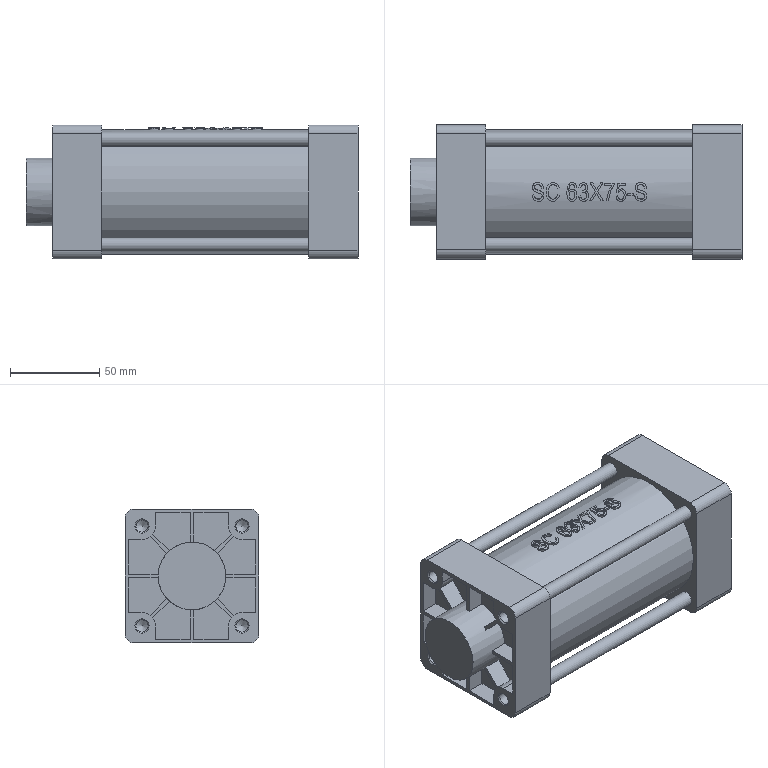Part | STEP file | Tube feed_id526_x_t | 1 solid | 220 faces | box 186 x 75 x 75 mm | volume 733898 mm3 | plane 109 | cylinder 56 | spline 39 | cone 16 | commonest cylinder face diameters 15 x16 38 x9 72 x9 6.8 x8 10 x8 8 x4